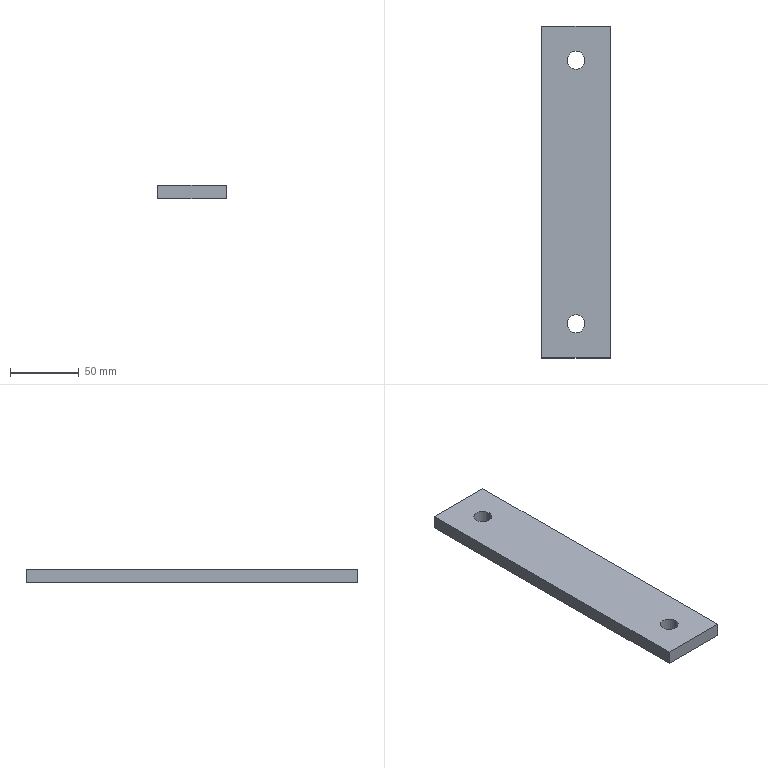Part | SolidWorks | features BaseBody 1 | 1 solid | 10 faces | box 50 x 242 x 10 mm | volume 118345 mm3 | plane 6 | cylinder 4 | commonest cylinder face diameters 13 x4
STEP:
#1=CARTESIAN_POINT('',(1486.5,496.,-25.));
#2=VERTEX_POINT('',#1);
#3=CARTESIAN_POINT('',(1473.5,496.,-25.));
#4=VERTEX_POINT('',#3);
#5=CARTESIAN_POINT('',(1480.,496.,-25.));
#6=DIRECTION('',(0.,0.,-1.));
#7=DIRECTION('',(-1.,0.,0.));
#8=AXIS2_PLACEMENT_3D('',#5,#6,#7);
#9=CIRCLE('',#8,6.5);
#10=EDGE_CURVE('',#2,#4,#9,.T.);
#11=ORIENTED_EDGE('',*,*,#10,.F.);
#12=CARTESIAN_POINT('',(1486.5,496.,-35.));
#13=VERTEX_POINT('',#12);
#14=CARTESIAN_POINT('',(1486.5,496.,-35.));
#15=DIRECTION('',(0.,0.,-1.));
#16=VECTOR('',#15,1000.);
#17=LINE('',#14,#16);
#18=EDGE_CURVE('',#2,#13,#17,.T.);
#19=ORIENTED_EDGE('',*,*,#18,.T.);
#20=CARTESIAN_POINT('',(1473.5,496.,-35.));
#21=VERTEX_POINT('',#20);
#22=CARTESIAN_POINT('',(1480.,496.,-35.));
#23=DIRECTION('',(0.,0.,-1.));
#24=DIRECTION('',(-1.,0.,0.));
#25=AXIS2_PLACEMENT_3D('',#22,#23,#24);
#26=CIRCLE('',#25,6.5);
#27=EDGE_CURVE('',#13,#21,#26,.T.);
#28=ORIENTED_EDGE('',*,*,#27,.T.);
#29=CARTESIAN_POINT('',(1473.5,496.,-35.));
#30=DIRECTION('',(0.,0.,-1.));
#31=VECTOR('',#30,1000.);
#32=LINE('',#29,#31);
#33=EDGE_CURVE('',#4,#21,#32,.T.);
#34=ORIENTED_EDGE('',*,*,#33,.F.);
#35=EDGE_LOOP('',(#11,#19,#28,#34));
#36=FACE_OUTER_BOUND('',#35,.T.);
#37=CARTESIAN_POINT('',(1480.,496.,-35.));
#38=DIRECTION('',(0.,0.,-1.));
#39=DIRECTION('',(-1.,0.,0.));
#40=AXIS2_PLACEMENT_3D('',#37,#38,#39);
#41=CYLINDRICAL_SURFACE('',#40,6.5);
#42=ADVANCED_FACE('',(#36),#41,.F.);
#43=CARTESIAN_POINT('',(1486.5,688.,-25.));
#44=VERTEX_POINT('',#43);
#45=CARTESIAN_POINT('',(1473.5,688.,-25.));
#46=VERTEX_POINT('',#45);
#47=CARTESIAN_POINT('',(1480.,688.,-25.));
#48=DIRECTION('',(0.,0.,-1.));
#49=DIRECTION('',(-1.,0.,0.));
#50=AXIS2_PLACEMENT_3D('',#47,#48,#49);
#51=CIRCLE('',#50,6.5);
#52=EDGE_CURVE('',#44,#46,#51,.T.);
#53=ORIENTED_EDGE('',*,*,#52,.F.);
#54=CARTESIAN_POINT('',(1486.5,688.,-35.));
#55=VERTEX_POINT('',#54);
#56=CARTESIAN_POINT('',(1486.5,688.,-35.));
#57=DIRECTION('',(0.,0.,-1.));
#58=VECTOR('',#57,1000.);
#59=LINE('',#56,#58);
#60=EDGE_CURVE('',#44,#55,#59,.T.);
#61=ORIENTED_EDGE('',*,*,#60,.T.);
#62=CARTESIAN_POINT('',(1473.5,688.,-35.));
#63=VERTEX_POINT('',#62);
#64=CARTESIAN_POINT('',(1480.,688.,-35.));
#65=DIRECTION('',(0.,0.,-1.));
#66=DIRECTION('',(-1.,0.,0.));
#67=AXIS2_PLACEMENT_3D('',#64,#65,#66);
#68=CIRCLE('',#67,6.5);
#69=EDGE_CURVE('',#55,#63,#68,.T.);
#70=ORIENTED_EDGE('',*,*,#69,.T.);
#71=CARTESIAN_POINT('',(1473.5,688.,-35.));
#72=DIRECTION('',(0.,0.,-1.));
#73=VECTOR('',#72,1000.);
#74=LINE('',#71,#73);
#75=EDGE_CURVE('',#46,#63,#74,.T.);
#76=ORIENTED_EDGE('',*,*,#75,.F.);
#77=EDGE_LOOP('',(#53,#61,#70,#76));
#78=FACE_OUTER_BOUND('',#77,.T.);
#79=CARTESIAN_POINT('',(1480.,688.,-35.));
#80=DIRECTION('',(0.,0.,-1.));
#81=DIRECTION('',(-1.,0.,0.));
#82=AXIS2_PLACEMENT_3D('',#79,#80,#81);
#83=CYLINDRICAL_SURFACE('',#82,6.5);
#84=ADVANCED_FACE('',(#78),#83,.F.);
#85=CARTESIAN_POINT('',(1480.,688.,-25.));
#86=DIRECTION('',(0.,0.,-1.));
#87=DIRECTION('',(-1.,0.,0.));
#88=AXIS2_PLACEMENT_3D('',#85,#86,#87);
#89=CIRCLE('',#88,6.5);
#90=EDGE_CURVE('',#46,#44,#89,.T.);
#91=ORIENTED_EDGE('',*,*,#90,.T.);
#92=ORIENTED_EDGE('',*,*,#52,.T.);
#93=EDGE_LOOP('',(#91,#92));
#94=FACE_BOUND('',#93,.T.);
#95=CARTESIAN_POINT('',(1480.,496.,-25.));
#96=DIRECTION('',(0.,0.,-1.));
#97=DIRECTION('',(-1.,0.,0.));
#98=AXIS2_PLACEMENT_3D('',#95,#96,#97);
#99=CIRCLE('',#98,6.5);
#100=EDGE_CURVE('',#4,#2,#99,.T.);
#101=ORIENTED_EDGE('',*,*,#100,.T.);
#102=ORIENTED_EDGE('',*,*,#10,.T.);
#103=EDGE_LOOP('',(#101,#102));
#104=FACE_BOUND('',#103,.T.);
#105=CARTESIAN_POINT('',(1455.,713.,-25.));
#106=VERTEX_POINT('',#105);
#107=CARTESIAN_POINT('',(1505.,713.,-25.));
#108=VERTEX_POINT('',#107);
#109=CARTESIAN_POINT('',(1455.,713.,-25.));
#110=DIRECTION('',(1.,0.,0.));
#111=VECTOR('',#110,1000.);
#112=LINE('',#109,#111);
#113=EDGE_CURVE('',#106,#108,#112,.T.);
#114=ORIENTED_EDGE('',*,*,#113,.F.);
#115=CARTESIAN_POINT('',(1455.,471.,-25.));
#116=VERTEX_POINT('',#115);
#117=CARTESIAN_POINT('',(1455.,675.,-25.));
#118=DIRECTION('',(0.,-1.,0.));
#119=VECTOR('',#118,1000.);
#120=LINE('',#117,#119);
#121=EDGE_CURVE('',#106,#116,#120,.T.);
#122=ORIENTED_EDGE('',*,*,#121,.T.);
#123=CARTESIAN_POINT('',(1505.,471.,-25.));
#124=VERTEX_POINT('',#123);
#125=CARTESIAN_POINT('',(1455.,471.,-25.));
#126=DIRECTION('',(1.,0.,0.));
#127=VECTOR('',#126,1000.);
#128=LINE('',#125,#127);
#129=EDGE_CURVE('',#116,#124,#128,.T.);
#130=ORIENTED_EDGE('',*,*,#129,.T.);
#131=CARTESIAN_POINT('',(1505.,675.,-25.));
#132=DIRECTION('',(0.,-1.,0.));
#133=VECTOR('',#132,1000.);
#134=LINE('',#131,#133);
#135=EDGE_CURVE('',#108,#124,#134,.T.);
#136=ORIENTED_EDGE('',*,*,#135,.F.);
#137=EDGE_LOOP('',(#114,#122,#130,#136));
#138=FACE_OUTER_BOUND('',#137,.T.);
#139=CARTESIAN_POINT('',(1480.,-100.,-25.));
#140=DIRECTION('',(0.,0.,-1.));
#141=DIRECTION('',(0.,-1.,0.));
#142=AXIS2_PLACEMENT_3D('',#139,#140,#141);
#143=PLANE('',#142);
#144=ADVANCED_FACE('',(#94,#104,#138),#143,.F.);
#145=CARTESIAN_POINT('',(1480.,688.,-35.));
#146=DIRECTION('',(0.,0.,-1.));
#147=DIRECTION('',(-1.,0.,0.));
#148=AXIS2_PLACEMENT_3D('',#145,#146,#147);
#149=CIRCLE('',#148,6.5);
#150=EDGE_CURVE('',#63,#55,#149,.T.);
#151=ORIENTED_EDGE('',*,*,#150,.F.);
#152=ORIENTED_EDGE('',*,*,#69,.F.);
#153=EDGE_LOOP('',(#151,#152));
#154=FACE_BOUND('',#153,.T.);
#155=CARTESIAN_POINT('',(1480.,496.,-35.));
#156=DIRECTION('',(0.,0.,-1.));
#157=DIRECTION('',(-1.,0.,0.));
#158=AXIS2_PLACEMENT_3D('',#155,#156,#157);
#159=CIRCLE('',#158,6.5);
#160=EDGE_CURVE('',#21,#13,#159,.T.);
#161=ORIENTED_EDGE('',*,*,#160,.F.);
#162=ORIENTED_EDGE('',*,*,#27,.F.);
#163=EDGE_LOOP('',(#161,#162));
#164=FACE_BOUND('',#163,.T.);
#165=CARTESIAN_POINT('',(1455.,713.,-35.));
#166=VERTEX_POINT('',#165);
#167=CARTESIAN_POINT('',(1505.,713.,-35.));
#168=VERTEX_POINT('',#167);
#169=CARTESIAN_POINT('',(1455.,713.,-35.));
#170=DIRECTION('',(1.,0.,0.));
#171=VECTOR('',#170,1000.);
#172=LINE('',#169,#171);
#173=EDGE_CURVE('',#166,#168,#172,.T.);
#174=ORIENTED_EDGE('',*,*,#173,.T.);
#175=CARTESIAN_POINT('',(1505.,471.,-35.));
#176=VERTEX_POINT('',#175);
#177=CARTESIAN_POINT('',(1505.,675.,-35.));
#178=DIRECTION('',(0.,-1.,0.));
#179=VECTOR('',#178,1000.);
#180=LINE('',#177,#179);
#181=EDGE_CURVE('',#168,#176,#180,.T.);
#182=ORIENTED_EDGE('',*,*,#181,.T.);
#183=CARTESIAN_POINT('',(1455.,471.,-35.));
#184=VERTEX_POINT('',#183);
#185=CARTESIAN_POINT('',(1455.,471.,-35.));
#186=DIRECTION('',(1.,0.,0.));
#187=VECTOR('',#186,1000.);
#188=LINE('',#185,#187);
#189=EDGE_CURVE('',#184,#176,#188,.T.);
#190=ORIENTED_EDGE('',*,*,#189,.F.);
#191=CARTESIAN_POINT('',(1455.,675.,-35.));
#192=DIRECTION('',(0.,-1.,0.));
#193=VECTOR('',#192,1000.);
#194=LINE('',#191,#193);
#195=EDGE_CURVE('',#166,#184,#194,.T.);
#196=ORIENTED_EDGE('',*,*,#195,.F.);
#197=EDGE_LOOP('',(#174,#182,#190,#196));
#198=FACE_OUTER_BOUND('',#197,.T.);
#199=CARTESIAN_POINT('',(1480.,-100.,-35.));
#200=DIRECTION('',(0.,0.,-1.));
#201=DIRECTION('',(0.,-1.,0.));
#202=AXIS2_PLACEMENT_3D('',#199,#200,#201);
#203=PLANE('',#202);
#204=ADVANCED_FACE('',(#154,#164,#198),#203,.T.);
#205=ORIENTED_EDGE('',*,*,#121,.F.);
#206=CARTESIAN_POINT('',(1455.,713.,-35.));
#207=DIRECTION('',(0.,0.,1.));
#208=VECTOR('',#207,1000.);
#209=LINE('',#206,#208);
#210=EDGE_CURVE('',#166,#106,#209,.T.);
#211=ORIENTED_EDGE('',*,*,#210,.F.);
#212=ORIENTED_EDGE('',*,*,#195,.T.);
#213=CARTESIAN_POINT('',(1455.,471.,-35.));
#214=DIRECTION('',(0.,0.,1.));
#215=VECTOR('',#214,1000.);
#216=LINE('',#213,#215);
#217=EDGE_CURVE('',#184,#116,#216,.T.);
#218=ORIENTED_EDGE('',*,*,#217,.T.);
#219=EDGE_LOOP('',(#205,#211,#212,#218));
#220=FACE_OUTER_BOUND('',#219,.T.);
#221=CARTESIAN_POINT('',(1455.,675.,-35.));
#222=DIRECTION('',(-1.,0.,0.));
#223=DIRECTION('',(0.,0.,1.));
#224=AXIS2_PLACEMENT_3D('',#221,#222,#223);
#225=PLANE('',#224);
#226=ADVANCED_FACE('',(#220),#225,.T.);
#227=ORIENTED_EDGE('',*,*,#129,.F.);
#228=ORIENTED_EDGE('',*,*,#217,.F.);
#229=ORIENTED_EDGE('',*,*,#189,.T.);
#230=CARTESIAN_POINT('',(1505.,471.,-35.));
#231=DIRECTION('',(0.,0.,1.));
#232=VECTOR('',#231,1000.);
#233=LINE('',#230,#232);
#234=EDGE_CURVE('',#176,#124,#233,.T.);
#235=ORIENTED_EDGE('',*,*,#234,.T.);
#236=EDGE_LOOP('',(#227,#228,#229,#235));
#237=FACE_OUTER_BOUND('',#236,.T.);
#238=CARTESIAN_POINT('',(1455.,471.,-35.));
#239=DIRECTION('',(0.,-1.,0.));
#240=DIRECTION('',(0.,0.,-1.));
#241=AXIS2_PLACEMENT_3D('',#238,#239,#240);
#242=PLANE('',#241);
#243=ADVANCED_FACE('',(#237),#242,.T.);
#244=ORIENTED_EDGE('',*,*,#135,.T.);
#245=ORIENTED_EDGE('',*,*,#234,.F.);
#246=ORIENTED_EDGE('',*,*,#181,.F.);
#247=CARTESIAN_POINT('',(1505.,713.,-35.));
#248=DIRECTION('',(0.,0.,1.));
#249=VECTOR('',#248,1000.);
#250=LINE('',#247,#249);
#251=EDGE_CURVE('',#168,#108,#250,.T.);
#252=ORIENTED_EDGE('',*,*,#251,.T.);
#253=EDGE_LOOP('',(#244,#245,#246,#252));
#254=FACE_OUTER_BOUND('',#253,.T.);
#255=CARTESIAN_POINT('',(1505.,675.,-35.));
#256=DIRECTION('',(-1.,0.,0.));
#257=DIRECTION('',(0.,0.,1.));
#258=AXIS2_PLACEMENT_3D('',#255,#256,#257);
#259=PLANE('',#258);
#260=ADVANCED_FACE('',(#254),#259,.F.);
#261=ORIENTED_EDGE('',*,*,#113,.T.);
#262=ORIENTED_EDGE('',*,*,#251,.F.);
#263=ORIENTED_EDGE('',*,*,#173,.F.);
#264=ORIENTED_EDGE('',*,*,#210,.T.);
#265=EDGE_LOOP('',(#261,#262,#263,#264));
#266=FACE_OUTER_BOUND('',#265,.T.);
#267=CARTESIAN_POINT('',(1455.,713.,-35.));
#268=DIRECTION('',(0.,-1.,0.));
#269=DIRECTION('',(0.,0.,-1.));
#270=AXIS2_PLACEMENT_3D('',#267,#268,#269);
#271=PLANE('',#270);
#272=ADVANCED_FACE('',(#266),#271,.F.);
#273=ORIENTED_EDGE('',*,*,#60,.F.);
#274=ORIENTED_EDGE('',*,*,#90,.F.);
#275=ORIENTED_EDGE('',*,*,#75,.T.);
#276=ORIENTED_EDGE('',*,*,#150,.T.);
#277=EDGE_LOOP('',(#273,#274,#275,#276));
#278=FACE_OUTER_BOUND('',#277,.T.);
#279=CARTESIAN_POINT('',(1480.,688.,-35.));
#280=DIRECTION('',(0.,0.,-1.));
#281=DIRECTION('',(-1.,0.,0.));
#282=AXIS2_PLACEMENT_3D('',#279,#280,#281);
#283=CYLINDRICAL_SURFACE('',#282,6.5);
#284=ADVANCED_FACE('',(#278),#283,.F.);
#285=ORIENTED_EDGE('',*,*,#18,.F.);
#286=ORIENTED_EDGE('',*,*,#100,.F.);
#287=ORIENTED_EDGE('',*,*,#33,.T.);
#288=ORIENTED_EDGE('',*,*,#160,.T.);
#289=EDGE_LOOP('',(#285,#286,#287,#288));
#290=FACE_OUTER_BOUND('',#289,.T.);
#291=CARTESIAN_POINT('',(1480.,496.,-35.));
#292=DIRECTION('',(0.,0.,-1.));
#293=DIRECTION('',(-1.,0.,0.));
#294=AXIS2_PLACEMENT_3D('',#291,#292,#293);
#295=CYLINDRICAL_SURFACE('',#294,6.5);
#296=ADVANCED_FACE('',(#290),#295,.F.);
#297=CLOSED_SHELL('',(#42,#84,#144,#204,#226,#243,#260,#272,#284,#296));
#298=MANIFOLD_SOLID_BREP('',#297);
#299=CARTESIAN_POINT('',(0.,0.,0.));
#300=DIRECTION('',(0.,0.,1.));
#301=DIRECTION('',(1.,0.,0.));
#302=AXIS2_PLACEMENT_3D('',#299,#300,#301);
#303=(LENGTH_UNIT()NAMED_UNIT(*)SI_UNIT(.MILLI.,.METRE.));
#304=UNCERTAINTY_MEASURE_WITH_UNIT(LENGTH_MEASURE(0.00001),#303,'','');
#305=(NAMED_UNIT(*)PLANE_ANGLE_UNIT()SI_UNIT($,.RADIAN.));
#306=(NAMED_UNIT(*)SI_UNIT($,.STERADIAN.)SOLID_ANGLE_UNIT());
#307=(GEOMETRIC_REPRESENTATION_CONTEXT(3)GLOBAL_UNCERTAINTY_ASSIGNED_CONTEXT((#304))GLOBAL_UNIT_ASSIGNED_CONTEXT((#303,#305,#306))REPRESENTATION_CONTEXT('',''));
#308=ADVANCED_BREP_SHAPE_REPRESENTATION('',(#298,#302),#307);